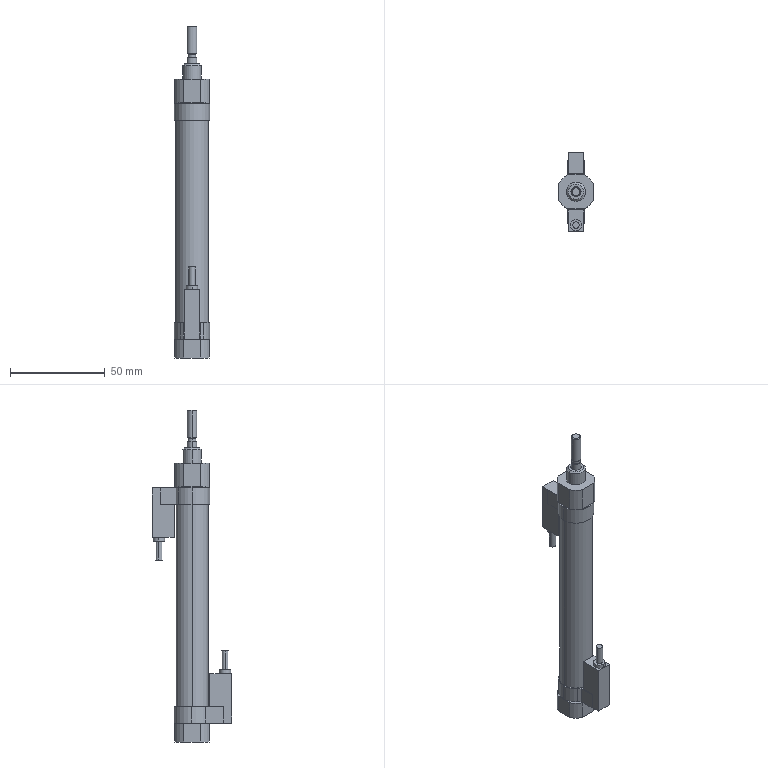Part | STEP file | Mount electronic clip sCDJ2B16-100-C73 | 3 solids | 113 faces | box 18.6 x 41.8 x 175 mm | volume 45989 mm3 | plane 53 | cylinder 46 | cone 10 | spline 4 | commonest cylinder face diameters 18.6 x8 20 x8 17.4 x6 3.4 x4 4.13 x4 5 x4